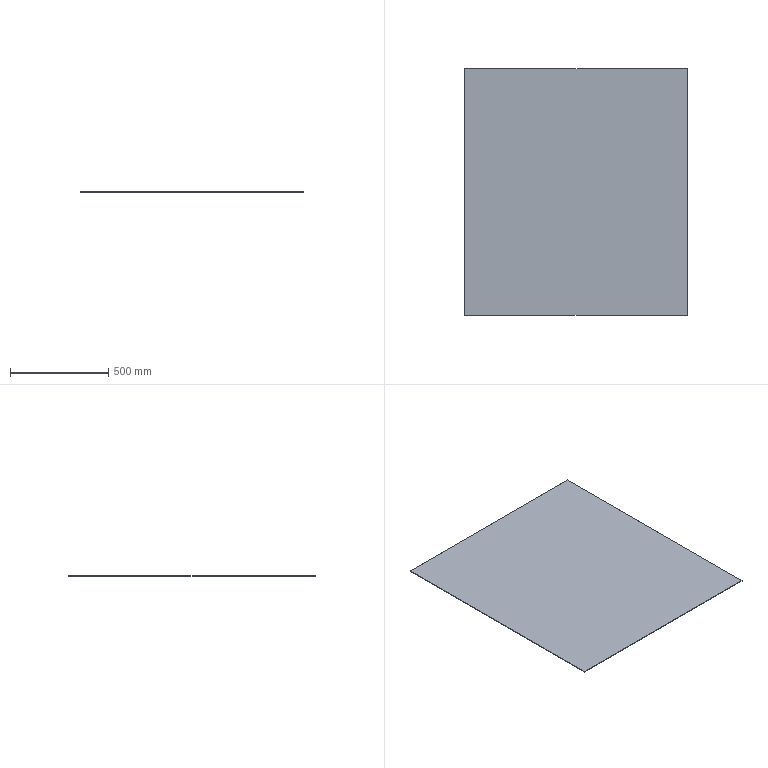Part | SolidWorks | features Extrusion 1 | 1 solid | 6 faces | box 1135 x 1255 x 3 mm | volume 4273275 mm3 | plane 6
STEP:
#1=CARTESIAN_POINT('',(567.5,-627.5,0.));
#2=VERTEX_POINT('',#1);
#3=CARTESIAN_POINT('',(567.5,627.5,0.));
#4=VERTEX_POINT('',#3);
#5=CARTESIAN_POINT('',(567.5,627.5,0.));
#6=DIRECTION('',(0.,1.,0.));
#7=VECTOR('',#6,1000.);
#8=LINE('',#5,#7);
#9=EDGE_CURVE('',#2,#4,#8,.T.);
#10=ORIENTED_EDGE('',*,*,#9,.T.);
#11=CARTESIAN_POINT('',(567.5,627.5,3.));
#12=VERTEX_POINT('',#11);
#13=CARTESIAN_POINT('',(567.5,627.5,3.));
#14=DIRECTION('',(0.,0.,-1.));
#15=VECTOR('',#14,1000.);
#16=LINE('',#13,#15);
#17=EDGE_CURVE('',#12,#4,#16,.T.);
#18=ORIENTED_EDGE('',*,*,#17,.F.);
#19=CARTESIAN_POINT('',(567.5,-627.5,3.));
#20=VERTEX_POINT('',#19);
#21=CARTESIAN_POINT('',(567.5,627.5,3.));
#22=DIRECTION('',(0.,1.,0.));
#23=VECTOR('',#22,1000.);
#24=LINE('',#21,#23);
#25=EDGE_CURVE('',#20,#12,#24,.T.);
#26=ORIENTED_EDGE('',*,*,#25,.F.);
#27=CARTESIAN_POINT('',(567.5,-627.5,3.));
#28=DIRECTION('',(0.,0.,-1.));
#29=VECTOR('',#28,1000.);
#30=LINE('',#27,#29);
#31=EDGE_CURVE('',#20,#2,#30,.T.);
#32=ORIENTED_EDGE('',*,*,#31,.T.);
#33=EDGE_LOOP('',(#10,#18,#26,#32));
#34=FACE_OUTER_BOUND('',#33,.T.);
#35=CARTESIAN_POINT('',(567.5,627.5,3.));
#36=DIRECTION('',(-1.,0.,0.));
#37=DIRECTION('',(0.,-1.,0.));
#38=AXIS2_PLACEMENT_3D('',#35,#36,#37);
#39=PLANE('',#38);
#40=ADVANCED_FACE('',(#34),#39,.F.);
#41=CARTESIAN_POINT('',(-567.5,627.5,0.));
#42=VERTEX_POINT('',#41);
#43=CARTESIAN_POINT('',(-567.5,627.5,0.));
#44=DIRECTION('',(-1.,0.,0.));
#45=VECTOR('',#44,1000.);
#46=LINE('',#43,#45);
#47=EDGE_CURVE('',#4,#42,#46,.T.);
#48=ORIENTED_EDGE('',*,*,#47,.T.);
#49=CARTESIAN_POINT('',(-567.5,627.5,3.));
#50=VERTEX_POINT('',#49);
#51=CARTESIAN_POINT('',(-567.5,627.5,3.));
#52=DIRECTION('',(0.,0.,-1.));
#53=VECTOR('',#52,1000.);
#54=LINE('',#51,#53);
#55=EDGE_CURVE('',#50,#42,#54,.T.);
#56=ORIENTED_EDGE('',*,*,#55,.F.);
#57=CARTESIAN_POINT('',(-567.5,627.5,3.));
#58=DIRECTION('',(-1.,0.,0.));
#59=VECTOR('',#58,1000.);
#60=LINE('',#57,#59);
#61=EDGE_CURVE('',#12,#50,#60,.T.);
#62=ORIENTED_EDGE('',*,*,#61,.F.);
#63=ORIENTED_EDGE('',*,*,#17,.T.);
#64=EDGE_LOOP('',(#48,#56,#62,#63));
#65=FACE_OUTER_BOUND('',#64,.T.);
#66=CARTESIAN_POINT('',(-567.5,627.5,3.));
#67=DIRECTION('',(0.,-1.,0.));
#68=DIRECTION('',(0.,0.,-1.));
#69=AXIS2_PLACEMENT_3D('',#66,#67,#68);
#70=PLANE('',#69);
#71=ADVANCED_FACE('',(#65),#70,.F.);
#72=CARTESIAN_POINT('',(-567.5,-627.5,0.));
#73=VERTEX_POINT('',#72);
#74=CARTESIAN_POINT('',(-567.5,627.5,0.));
#75=DIRECTION('',(0.,-1.,0.));
#76=VECTOR('',#75,1000.);
#77=LINE('',#74,#76);
#78=EDGE_CURVE('',#42,#73,#77,.T.);
#79=ORIENTED_EDGE('',*,*,#78,.T.);
#80=CARTESIAN_POINT('',(-567.5,-627.5,3.));
#81=VERTEX_POINT('',#80);
#82=CARTESIAN_POINT('',(-567.5,-627.5,3.));
#83=DIRECTION('',(0.,0.,-1.));
#84=VECTOR('',#83,1000.);
#85=LINE('',#82,#84);
#86=EDGE_CURVE('',#81,#73,#85,.T.);
#87=ORIENTED_EDGE('',*,*,#86,.F.);
#88=CARTESIAN_POINT('',(-567.5,627.5,3.));
#89=DIRECTION('',(0.,-1.,0.));
#90=VECTOR('',#89,1000.);
#91=LINE('',#88,#90);
#92=EDGE_CURVE('',#50,#81,#91,.T.);
#93=ORIENTED_EDGE('',*,*,#92,.F.);
#94=ORIENTED_EDGE('',*,*,#55,.T.);
#95=EDGE_LOOP('',(#79,#87,#93,#94));
#96=FACE_OUTER_BOUND('',#95,.T.);
#97=CARTESIAN_POINT('',(-567.5,627.5,3.));
#98=DIRECTION('',(1.,0.,0.));
#99=DIRECTION('',(0.,0.,-1.));
#100=AXIS2_PLACEMENT_3D('',#97,#98,#99);
#101=PLANE('',#100);
#102=ADVANCED_FACE('',(#96),#101,.F.);
#103=CARTESIAN_POINT('',(-567.5,-627.5,0.));
#104=DIRECTION('',(1.,0.,0.));
#105=VECTOR('',#104,1000.);
#106=LINE('',#103,#105);
#107=EDGE_CURVE('',#73,#2,#106,.T.);
#108=ORIENTED_EDGE('',*,*,#107,.T.);
#109=ORIENTED_EDGE('',*,*,#31,.F.);
#110=CARTESIAN_POINT('',(-567.5,-627.5,3.));
#111=DIRECTION('',(1.,0.,0.));
#112=VECTOR('',#111,1000.);
#113=LINE('',#110,#112);
#114=EDGE_CURVE('',#81,#20,#113,.T.);
#115=ORIENTED_EDGE('',*,*,#114,.F.);
#116=ORIENTED_EDGE('',*,*,#86,.T.);
#117=EDGE_LOOP('',(#108,#109,#115,#116));
#118=FACE_OUTER_BOUND('',#117,.T.);
#119=CARTESIAN_POINT('',(-567.5,-627.5,3.));
#120=DIRECTION('',(0.,1.,0.));
#121=DIRECTION('',(0.,0.,1.));
#122=AXIS2_PLACEMENT_3D('',#119,#120,#121);
#123=PLANE('',#122);
#124=ADVANCED_FACE('',(#118),#123,.F.);
#125=ORIENTED_EDGE('',*,*,#25,.T.);
#126=ORIENTED_EDGE('',*,*,#61,.T.);
#127=ORIENTED_EDGE('',*,*,#92,.T.);
#128=ORIENTED_EDGE('',*,*,#114,.T.);
#129=EDGE_LOOP('',(#125,#126,#127,#128));
#130=FACE_OUTER_BOUND('',#129,.T.);
#131=CARTESIAN_POINT('',(0.,0.,3.));
#132=DIRECTION('',(0.,0.,1.));
#133=DIRECTION('',(1.,0.,0.));
#134=AXIS2_PLACEMENT_3D('',#131,#132,#133);
#135=PLANE('',#134);
#136=ADVANCED_FACE('',(#130),#135,.T.);
#137=ORIENTED_EDGE('',*,*,#9,.F.);
#138=ORIENTED_EDGE('',*,*,#107,.F.);
#139=ORIENTED_EDGE('',*,*,#78,.F.);
#140=ORIENTED_EDGE('',*,*,#47,.F.);
#141=EDGE_LOOP('',(#137,#138,#139,#140));
#142=FACE_OUTER_BOUND('',#141,.T.);
#143=CARTESIAN_POINT('',(0.,0.,0.));
#144=DIRECTION('',(0.,0.,1.));
#145=DIRECTION('',(1.,0.,0.));
#146=AXIS2_PLACEMENT_3D('',#143,#144,#145);
#147=PLANE('',#146);
#148=ADVANCED_FACE('',(#142),#147,.F.);
#149=CLOSED_SHELL('',(#40,#71,#102,#124,#136,#148));
#150=MANIFOLD_SOLID_BREP('',#149);
#151=CARTESIAN_POINT('',(0.,0.,0.));
#152=DIRECTION('',(0.,0.,1.));
#153=DIRECTION('',(1.,0.,0.));
#154=AXIS2_PLACEMENT_3D('',#151,#152,#153);
#155=(LENGTH_UNIT()NAMED_UNIT(*)SI_UNIT(.MILLI.,.METRE.));
#156=UNCERTAINTY_MEASURE_WITH_UNIT(LENGTH_MEASURE(0.00001),#155,'','');
#157=(NAMED_UNIT(*)PLANE_ANGLE_UNIT()SI_UNIT($,.RADIAN.));
#158=(NAMED_UNIT(*)SI_UNIT($,.STERADIAN.)SOLID_ANGLE_UNIT());
#159=(GEOMETRIC_REPRESENTATION_CONTEXT(3)GLOBAL_UNCERTAINTY_ASSIGNED_CONTEXT((#156))GLOBAL_UNIT_ASSIGNED_CONTEXT((#155,#157,#158))REPRESENTATION_CONTEXT('',''));
#160=ADVANCED_BREP_SHAPE_REPRESENTATION('',(#150,#154),#159);